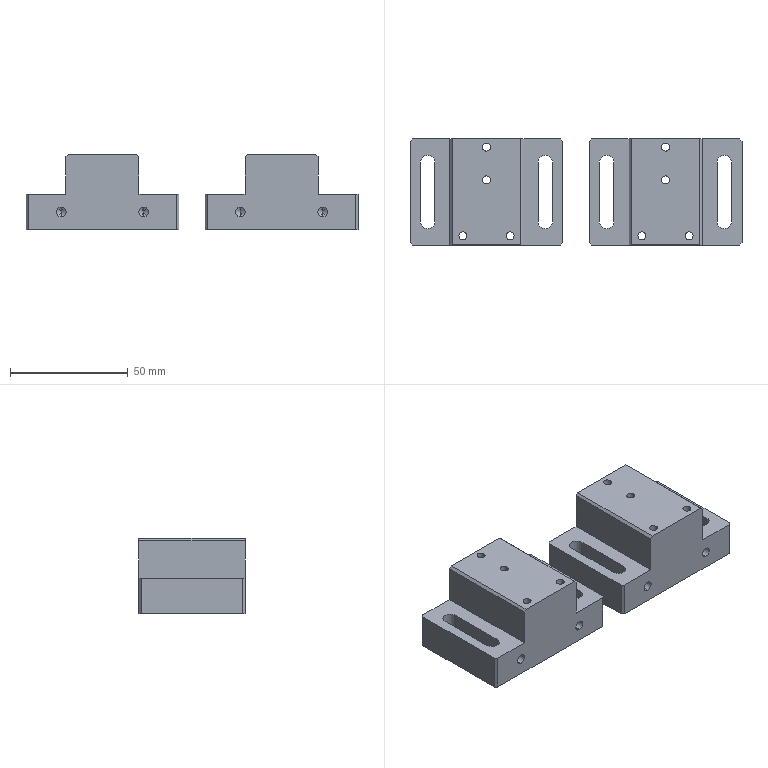NC program | NX | posted with a generic post | part box 140.92 x 45 x 32 mm
Lines 9989 to 10208 of 10208:
(DRILLING_COPY , TOOL : D6A45)
N19970 T01 M6
N19972 G54
N19974 G17 G0 G90 X108.46 Y3.5 S9500 M3
N19976 G43 Z30. H1
N19978 G94 G81 G98 Z-1.8 F250. R3.
N19980 Y17.4
N19982 X118.46 Y41.1
N19984 X98.46
N19986 X42.46
N19988 X22.46
N19990 X32.46 Y17.4
N19992 Y3.5
N19994 G80
N19996 G0 X32.46 Y3.5 Z30.
N19998 M5
(DRILLING_COPY_COPY_COPY , TOOL : 6.0ZT)
N20000 T17 M6
N20002 G54
N20004 G17 G0 G90 X108.46 Y3.5 S2000 M3
N20006 G43 Z30. H17
N20008 G94 G83 G98 Z-20.203 F150. Q2. R3.
N20010 Y17.4
N20012 X118.46 Y41.1
N20014 X98.46
N20016 X42.46
N20018 X22.46
N20020 X32.46 Y17.4
N20022 Y3.5
N20024 G80
N20026 G0 X32.46 Y3.5 Z30.
N20028 M5
(PLANAR_MILL_COPY_COPY_2 , TOOL : D6A45)
N20030 T01 M6
N20032 G54
N20034 G17 G0 G90 X31.594 Y1.9 S9500 M3
N20036 G43 Z30. H1
N20038 Z0.5
N20040 G94 G1 Z-1. F1250.
N20042 G3 X32.46 Y1.4 R1.
N20044 X34.56 Y3.5 R2.1
N20046 X32.46 Y1.4 R-2.1
N20048 X33.326 Y1.9 R1.
N20050 G1 Z0.5
N20052 G0 Z30.
N20054 X31.594 Y15.8
N20056 Z0.5
N20058 G1 Z-1.
N20060 G3 X32.46 Y15.3 R1.
N20062 X34.56 Y17.4 R2.1
N20064 X32.46 Y15.3 R-2.1
N20066 X33.326 Y15.8 R1.
N20068 G1 Z0.5
N20070 G0 Z30.
N20072 Y-1.4
N20074 Z0.5
N20076 G1 Z-1.
N20078 G3 X32.46 Y-0.9 R1.
N20080 G1 X0.96
N20082 G2 X0.324 Y-0.636 R0.9
N20084 G1 X-0.636 Y0.324
N20086 G2 X-0.9 Y0.96 R0.9
N20088 G1 Y44.04
N20090 G2 X-0.636 Y44.676 R0.9
N20092 G1 X0.324 Y45.636
N20094 G2 X0.96 Y45.9 R0.9
N20096 G1 X63.96
N20098 G2 X64.596 Y45.636 R0.9
N20100 G1 X65.556 Y44.676
N20102 G2 X65.82 Y44.04 R0.9
N20104 G1 Y0.96
N20106 G2 X65.556 Y0.324 R0.9
N20108 G1 X64.596 Y-0.636
N20110 G2 X63.96 Y-0.9 R0.9
N20112 G1 X32.46
N20114 G3 X31.594 Y-1.4 R1.
N20116 G1 Z0.5
N20118 G0 Z30.
N20120 X5.76 Y23.366
N20122 Z0.5
N20124 G1 Z-1.
N20126 G3 X5.26 Y22.5 R1.
N20128 G1 Y10.
N20130 G3 X7.46 Y7.8 R2.2
N20132 X9.66 Y10. R2.2
N20134 G1 Y35.
N20136 G3 X7.46 Y37.2 R2.2
N20138 X5.26 Y35. R2.2
N20140 G1 Y22.5
N20142 G3 X5.76 Y21.634 R1.
N20144 G1 Z0.5
N20146 G0 Z30.
N20148 X23.326 Y42.7
N20150 Z0.5
N20152 G1 Z-1.
N20154 G3 X22.46 Y43.2 R1.
N20156 X20.36 Y41.1 R2.1
N20158 X22.46 Y43.2 R-2.1
N20160 X21.594 Y42.7 R1.
N20162 G1 Z0.5
N20164 G0 Z30.
N20166 X43.326
N20168 Z0.5
N20170 G1 Z-1.
N20172 G3 X42.46 Y43.2 R1.
N20174 X40.36 Y41.1 R2.1
N20176 X42.46 Y43.2 R-2.1
N20178 X41.594 Y42.7 R1.
N20180 G1 Z0.5
N20182 G0 Z30.
N20184 X55.76 Y23.366
N20186 Z0.5
N20188 G1 Z-1.
N20190 G3 X55.26 Y22.5 R1.
N20192 G1 Y10.
N20194 G3 X57.46 Y7.8 R2.2
N20196 X59.66 Y10. R2.2
N20198 G1 Y35.
N20200 G3 X57.46 Y37.2 R2.2
N20202 X55.26 Y35. R2.2
N20204 G1 Y22.5
N20206 G3 X55.76 Y21.634 R1.
N20208 G1 Z0.5
N20210 G0 Z30.
N20212 X81.76 Y23.366
N20214 Z0.5
N20216 G1 Z-1.
N20218 G3 X81.26 Y22.5 R1.
N20220 G1 Y10.
N20222 G3 X83.46 Y7.8 R2.2
N20224 X85.66 Y10. R2.2
N20226 G1 Y35.
N20228 G3 X83.46 Y37.2 R2.2
N20230 X81.26 Y35. R2.2
N20232 G1 Y22.5
N20234 G3 X81.76 Y21.634 R1.
N20236 G1 Z0.5
N20238 G0 Z30.
N20240 X99.326 Y42.7
N20242 Z0.5
N20244 G1 Z-1.
N20246 G3 X98.46 Y43.2 R1.
N20248 X96.36 Y41.1 R2.1
N20250 X98.46 Y43.2 R-2.1
N20252 X97.594 Y42.7 R1.
N20254 G1 Z0.5
N20256 G0 Z30.
N20258 X119.326
N20260 Z0.5
N20262 G1 Z-1.
N20264 G3 X118.46 Y43.2 R1.
N20266 X116.36 Y41.1 R2.1
N20268 X118.46 Y43.2 R-2.1
N20270 X117.594 Y42.7 R1.
N20272 G1 Z0.5
N20274 G0 Z30.
N20276 X135.16 Y21.634
N20278 Z0.5
N20280 G1 Z-1.
N20282 G3 X135.66 Y22.5 R1.
N20284 G1 Y35.
N20286 G3 X133.46 Y37.2 R2.2
N20288 X131.26 Y35. R2.2
N20290 G1 Y10.
N20292 G3 X133.46 Y7.8 R2.2
N20294 X135.66 Y10. R2.2
N20296 G1 Y22.5
N20298 G3 X135.16 Y23.366 R1.
N20300 G1 Z0.5
N20302 G0 Z30.
N20304 X107.594 Y46.4
N20306 Z0.5
N20308 G1 Z-1.
N20310 G3 X108.46 Y45.9 R1.
N20312 G1 X139.96
N20314 G2 X140.596 Y45.636 R0.9
N20316 G1 X141.556 Y44.676
N20318 G2 X141.82 Y44.04 R0.9
N20320 G1 Y0.96
N20322 G2 X141.556 Y0.324 R0.9
N20324 G1 X140.596 Y-0.636
N20326 G2 X139.96 Y-0.9 R0.9
N20328 G1 X76.96
N20330 G2 X76.324 Y-0.636 R0.9
N20332 G1 X75.364 Y0.324
N20334 G2 X75.1 Y0.96 R0.9
N20336 G1 Y44.04
N20338 G2 X75.364 Y44.676 R0.9
N20340 G1 X76.324 Y45.636
N20342 G2 X76.96 Y45.9 R0.9
N20344 G1 X108.46
N20346 G3 X109.326 Y46.4 R1.
N20348 G1 Z0.5
N20350 G0 Z30.
N20352 X107.594 Y15.8
N20354 Z0.5
N20356 G1 Z-1.
N20358 G3 X108.46 Y15.3 R1.
N20360 X110.56 Y17.4 R2.1
N20362 X108.46 Y15.3 R-2.1
N20364 X109.326 Y15.8 R1.
N20366 G1 Z0.5
N20368 G0 Z30.
N20370 X107.594 Y1.9
N20372 Z0.5
N20374 G1 Z-1.
N20376 G3 X108.46 Y1.4 R1.
N20378 X110.56 Y3.5 R2.1
N20380 X108.46 Y1.4 R-2.1
N20382 X109.326 Y1.9 R1.
N20384 G1 Z0.5
N20386 G0 Z30.
N20388 M5
N20390 M2